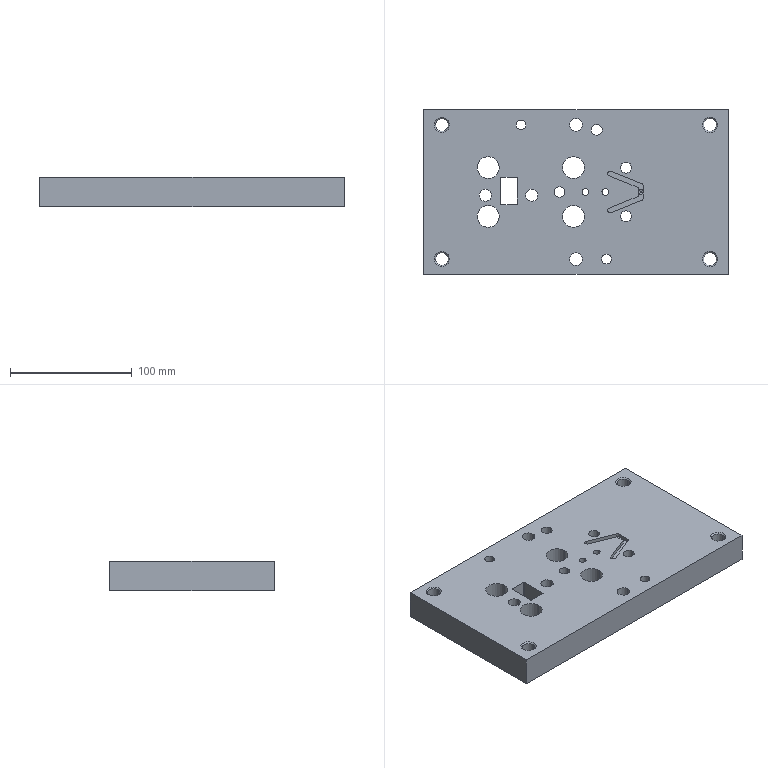Part | STEP file | MIENG DE KHUON DUONG CO LOGO | 1 solid | 128 faces | box 250 x 135 x 24 mm | volume 741333 mm3 | cylinder 73 | plane 33 | cone 22 | commonest cylinder face diameters 10.5 x12 4 x8 10 x8 18 x8 9 x6 15 x6